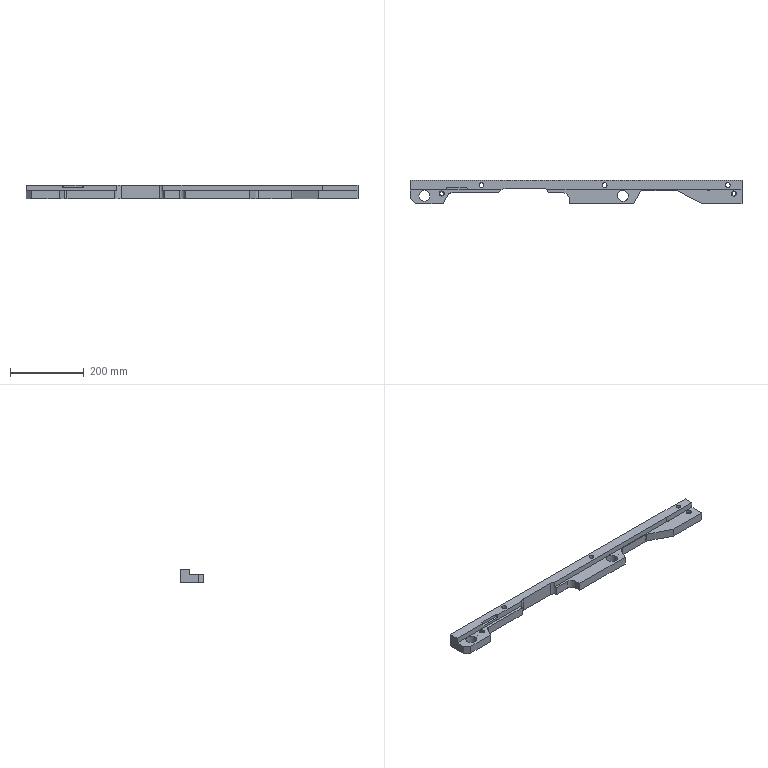Part | STEP file | gslz 2016.10.28-13_id994_x_t | 1 solid | 70 faces | box 903 x 64 x 38 mm | volume 1224228 mm3 | cylinder 29 | plane 29 | cone 12 | commonest cylinder face diameters 6.8 x6 5.2 x4 13 x3 18 x3 30 x3 6 x2